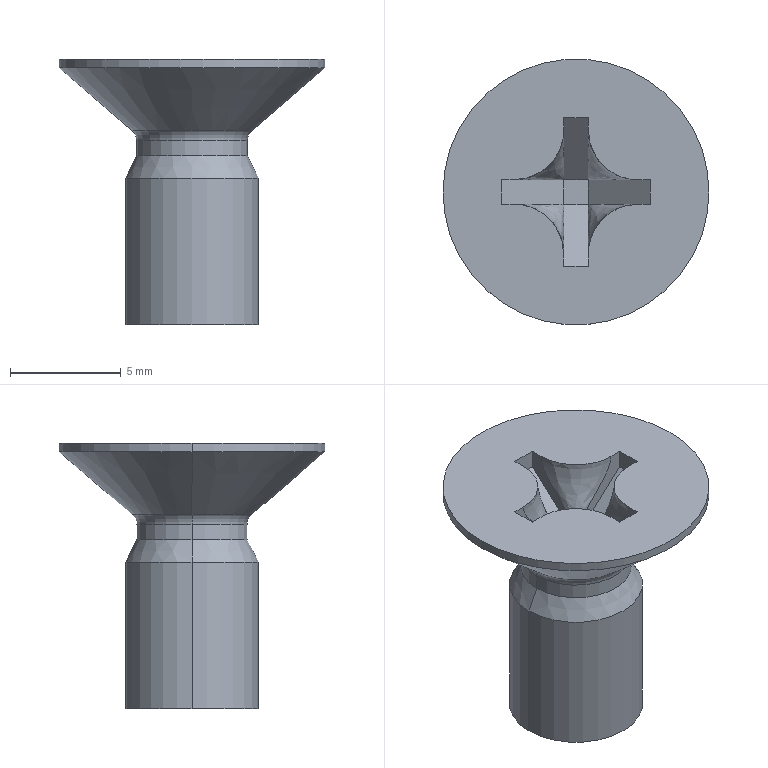Part | STEP file | 0217_305_SFBJ6-12 | 1 solid | 35 faces | box 12 x 12 x 12 mm | volume 419.433 mm3 | plane 19 | cylinder 6 | cone 4 | spline 4 | torus 2 | commonest cylinder face diameters 5 x2 6 x2 12 x2